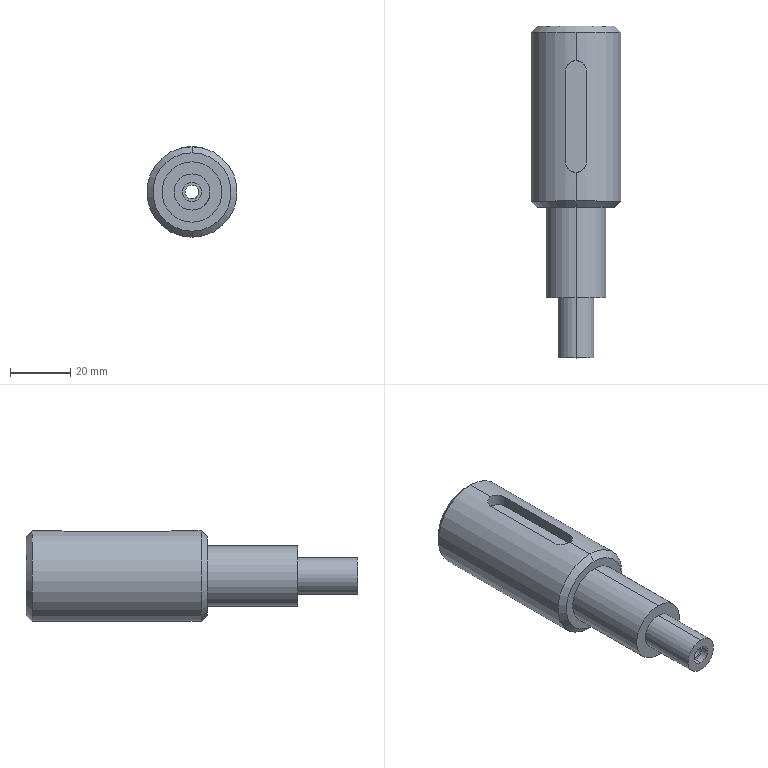Part | STEP file | BU-A13#130a | 1 solid | 43 faces | box 30 x 110 x 30 mm | volume 44972 mm3 | cylinder 22 | cone 11 | plane 10 | commonest cylinder face diameters 2.5 x4 4.2 x2 4.6 x2 6.3 x2 7 x2 9 x2